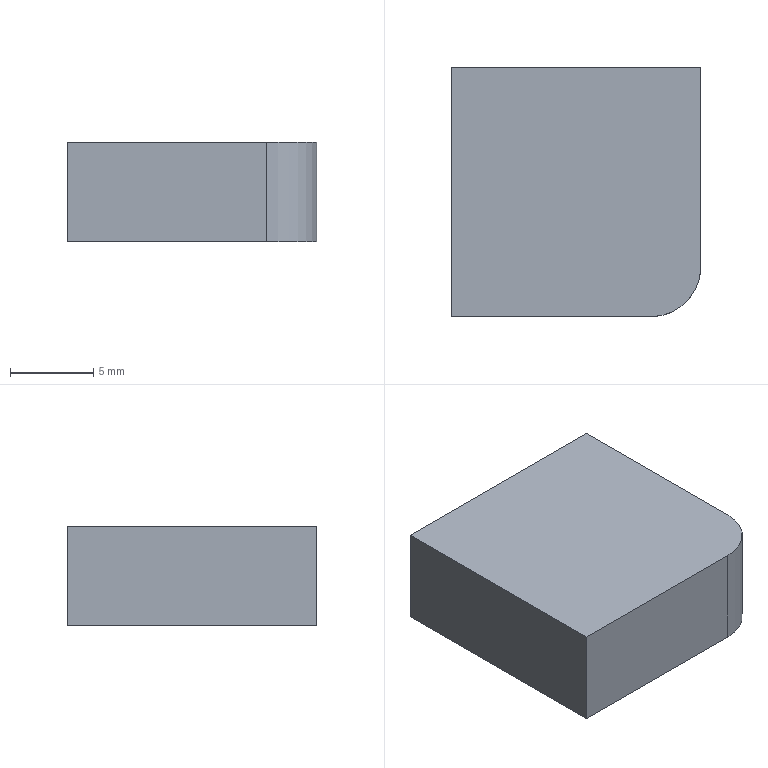Part | SolidWorks | features FlatPattern 1, SMBaseFlange 1, SheetMetal 1 | 1 solid | 7 faces | box 15 x 15 x 6 mm | volume 1338 mm3 | plane 6 | cylinder 1 | commonest cylinder face diameters 6 x1
STEP:
#1=CARTESIAN_POINT('',(675.3,-99.409,0.));
#2=VERTEX_POINT('',#1);
#3=CARTESIAN_POINT('',(675.3,-87.409,0.));
#4=VERTEX_POINT('',#3);
#5=CARTESIAN_POINT('',(675.3,-87.409,0.));
#6=DIRECTION('',(0.,1.,0.));
#7=VECTOR('',#6,1000.);
#8=LINE('',#5,#7);
#9=EDGE_CURVE('',#2,#4,#8,.T.);
#10=ORIENTED_EDGE('',*,*,#9,.F.);
#11=CARTESIAN_POINT('',(675.3,-99.409,-6.));
#12=VERTEX_POINT('',#11);
#13=CARTESIAN_POINT('',(675.3,-99.409,-6.));
#14=DIRECTION('',(0.,0.,1.));
#15=VECTOR('',#14,1000.);
#16=LINE('',#13,#15);
#17=EDGE_CURVE('',#12,#2,#16,.T.);
#18=ORIENTED_EDGE('',*,*,#17,.F.);
#19=CARTESIAN_POINT('',(675.3,-87.409,-6.));
#20=VERTEX_POINT('',#19);
#21=CARTESIAN_POINT('',(675.3,-87.409,-6.));
#22=DIRECTION('',(0.,1.,0.));
#23=VECTOR('',#22,1000.);
#24=LINE('',#21,#23);
#25=EDGE_CURVE('',#12,#20,#24,.T.);
#26=ORIENTED_EDGE('',*,*,#25,.T.);
#27=CARTESIAN_POINT('',(675.3,-87.409,-6.));
#28=DIRECTION('',(0.,0.,1.));
#29=VECTOR('',#28,1000.);
#30=LINE('',#27,#29);
#31=EDGE_CURVE('',#20,#4,#30,.T.);
#32=ORIENTED_EDGE('',*,*,#31,.T.);
#33=EDGE_LOOP('',(#10,#18,#26,#32));
#34=FACE_OUTER_BOUND('',#33,.T.);
#35=CARTESIAN_POINT('',(675.3,-87.409,-6.));
#36=DIRECTION('',(1.,0.,0.));
#37=DIRECTION('',(0.,0.,-1.));
#38=AXIS2_PLACEMENT_3D('',#35,#36,#37);
#39=PLANE('',#38);
#40=ADVANCED_FACE('',(#34),#39,.T.);
#41=CARTESIAN_POINT('',(672.3,-102.409,0.));
#42=VERTEX_POINT('',#41);
#43=CARTESIAN_POINT('',(672.3,-99.409,0.));
#44=DIRECTION('',(0.,0.,1.));
#45=DIRECTION('',(-1.,0.,0.));
#46=AXIS2_PLACEMENT_3D('',#43,#44,#45);
#47=CIRCLE('',#46,3.);
#48=EDGE_CURVE('',#42,#2,#47,.T.);
#49=ORIENTED_EDGE('',*,*,#48,.F.);
#50=CARTESIAN_POINT('',(672.3,-102.409,-6.));
#51=VERTEX_POINT('',#50);
#52=CARTESIAN_POINT('',(672.3,-102.409,-6.));
#53=DIRECTION('',(0.,0.,1.));
#54=VECTOR('',#53,1000.);
#55=LINE('',#52,#54);
#56=EDGE_CURVE('',#51,#42,#55,.T.);
#57=ORIENTED_EDGE('',*,*,#56,.F.);
#58=CARTESIAN_POINT('',(672.3,-99.409,-6.));
#59=DIRECTION('',(0.,0.,1.));
#60=DIRECTION('',(-1.,0.,0.));
#61=AXIS2_PLACEMENT_3D('',#58,#59,#60);
#62=CIRCLE('',#61,3.);
#63=EDGE_CURVE('',#51,#12,#62,.T.);
#64=ORIENTED_EDGE('',*,*,#63,.T.);
#65=ORIENTED_EDGE('',*,*,#17,.T.);
#66=EDGE_LOOP('',(#49,#57,#64,#65));
#67=FACE_OUTER_BOUND('',#66,.T.);
#68=CARTESIAN_POINT('',(672.3,-99.409,-6.));
#69=DIRECTION('',(0.,0.,1.));
#70=DIRECTION('',(1.,0.,0.));
#71=AXIS2_PLACEMENT_3D('',#68,#69,#70);
#72=CYLINDRICAL_SURFACE('',#71,3.);
#73=ADVANCED_FACE('',(#67),#72,.T.);
#74=CARTESIAN_POINT('',(660.3,-102.409,0.));
#75=VERTEX_POINT('',#74);
#76=CARTESIAN_POINT('',(672.3,-102.409,0.));
#77=DIRECTION('',(1.,0.,0.));
#78=VECTOR('',#77,1000.);
#79=LINE('',#76,#78);
#80=EDGE_CURVE('',#75,#42,#79,.T.);
#81=ORIENTED_EDGE('',*,*,#80,.F.);
#82=CARTESIAN_POINT('',(660.3,-102.409,-6.));
#83=VERTEX_POINT('',#82);
#84=CARTESIAN_POINT('',(660.3,-102.409,-6.));
#85=DIRECTION('',(0.,0.,1.));
#86=VECTOR('',#85,1000.);
#87=LINE('',#84,#86);
#88=EDGE_CURVE('',#83,#75,#87,.T.);
#89=ORIENTED_EDGE('',*,*,#88,.F.);
#90=CARTESIAN_POINT('',(672.3,-102.409,-6.));
#91=DIRECTION('',(1.,0.,0.));
#92=VECTOR('',#91,1000.);
#93=LINE('',#90,#92);
#94=EDGE_CURVE('',#83,#51,#93,.T.);
#95=ORIENTED_EDGE('',*,*,#94,.T.);
#96=ORIENTED_EDGE('',*,*,#56,.T.);
#97=EDGE_LOOP('',(#81,#89,#95,#96));
#98=FACE_OUTER_BOUND('',#97,.T.);
#99=CARTESIAN_POINT('',(672.3,-102.409,-6.));
#100=DIRECTION('',(0.,-1.,0.));
#101=DIRECTION('',(0.,0.,-1.));
#102=AXIS2_PLACEMENT_3D('',#99,#100,#101);
#103=PLANE('',#102);
#104=ADVANCED_FACE('',(#98),#103,.T.);
#105=CARTESIAN_POINT('',(660.3,-87.409,0.));
#106=VERTEX_POINT('',#105);
#107=CARTESIAN_POINT('',(660.3,-87.409,0.));
#108=DIRECTION('',(0.,-1.,0.));
#109=VECTOR('',#108,1000.);
#110=LINE('',#107,#109);
#111=EDGE_CURVE('',#106,#75,#110,.T.);
#112=ORIENTED_EDGE('',*,*,#111,.F.);
#113=CARTESIAN_POINT('',(660.3,-87.409,-6.));
#114=VERTEX_POINT('',#113);
#115=CARTESIAN_POINT('',(660.3,-87.409,-6.));
#116=DIRECTION('',(0.,0.,1.));
#117=VECTOR('',#116,1000.);
#118=LINE('',#115,#117);
#119=EDGE_CURVE('',#114,#106,#118,.T.);
#120=ORIENTED_EDGE('',*,*,#119,.F.);
#121=CARTESIAN_POINT('',(660.3,-87.409,-6.));
#122=DIRECTION('',(0.,-1.,0.));
#123=VECTOR('',#122,1000.);
#124=LINE('',#121,#123);
#125=EDGE_CURVE('',#114,#83,#124,.T.);
#126=ORIENTED_EDGE('',*,*,#125,.T.);
#127=ORIENTED_EDGE('',*,*,#88,.T.);
#128=EDGE_LOOP('',(#112,#120,#126,#127));
#129=FACE_OUTER_BOUND('',#128,.T.);
#130=CARTESIAN_POINT('',(660.3,-87.409,-6.));
#131=DIRECTION('',(-1.,0.,0.));
#132=DIRECTION('',(0.,-1.,0.));
#133=AXIS2_PLACEMENT_3D('',#130,#131,#132);
#134=PLANE('',#133);
#135=ADVANCED_FACE('',(#129),#134,.T.);
#136=CARTESIAN_POINT('',(675.3,-87.409,0.));
#137=DIRECTION('',(-1.,0.,0.));
#138=VECTOR('',#137,1000.);
#139=LINE('',#136,#138);
#140=EDGE_CURVE('',#4,#106,#139,.T.);
#141=ORIENTED_EDGE('',*,*,#140,.F.);
#142=ORIENTED_EDGE('',*,*,#31,.F.);
#143=CARTESIAN_POINT('',(675.3,-87.409,-6.));
#144=DIRECTION('',(-1.,0.,0.));
#145=VECTOR('',#144,1000.);
#146=LINE('',#143,#145);
#147=EDGE_CURVE('',#20,#114,#146,.T.);
#148=ORIENTED_EDGE('',*,*,#147,.T.);
#149=ORIENTED_EDGE('',*,*,#119,.T.);
#150=EDGE_LOOP('',(#141,#142,#148,#149));
#151=FACE_OUTER_BOUND('',#150,.T.);
#152=CARTESIAN_POINT('',(675.3,-87.409,-6.));
#153=DIRECTION('',(0.,1.,0.));
#154=DIRECTION('',(-1.,0.,0.));
#155=AXIS2_PLACEMENT_3D('',#152,#153,#154);
#156=PLANE('',#155);
#157=ADVANCED_FACE('',(#151),#156,.T.);
#158=ORIENTED_EDGE('',*,*,#25,.F.);
#159=ORIENTED_EDGE('',*,*,#63,.F.);
#160=ORIENTED_EDGE('',*,*,#94,.F.);
#161=ORIENTED_EDGE('',*,*,#125,.F.);
#162=ORIENTED_EDGE('',*,*,#147,.F.);
#163=EDGE_LOOP('',(#158,#159,#160,#161,#162));
#164=FACE_OUTER_BOUND('',#163,.T.);
#165=CARTESIAN_POINT('',(672.3,-99.409,-6.));
#166=DIRECTION('',(0.,0.,-1.));
#167=DIRECTION('',(-1.,0.,0.));
#168=AXIS2_PLACEMENT_3D('',#165,#166,#167);
#169=PLANE('',#168);
#170=ADVANCED_FACE('',(#164),#169,.T.);
#171=ORIENTED_EDGE('',*,*,#9,.T.);
#172=ORIENTED_EDGE('',*,*,#140,.T.);
#173=ORIENTED_EDGE('',*,*,#111,.T.);
#174=ORIENTED_EDGE('',*,*,#80,.T.);
#175=ORIENTED_EDGE('',*,*,#48,.T.);
#176=EDGE_LOOP('',(#171,#172,#173,#174,#175));
#177=FACE_OUTER_BOUND('',#176,.T.);
#178=CARTESIAN_POINT('',(672.3,-99.409,0.));
#179=DIRECTION('',(0.,0.,-1.));
#180=DIRECTION('',(-1.,0.,0.));
#181=AXIS2_PLACEMENT_3D('',#178,#179,#180);
#182=PLANE('',#181);
#183=ADVANCED_FACE('',(#177),#182,.F.);
#184=CLOSED_SHELL('',(#40,#73,#104,#135,#157,#170,#183));
#185=MANIFOLD_SOLID_BREP('',#184);
#186=CARTESIAN_POINT('',(0.,0.,0.));
#187=DIRECTION('',(0.,0.,1.));
#188=DIRECTION('',(1.,0.,0.));
#189=AXIS2_PLACEMENT_3D('',#186,#187,#188);
#190=(LENGTH_UNIT()NAMED_UNIT(*)SI_UNIT(.MILLI.,.METRE.));
#191=UNCERTAINTY_MEASURE_WITH_UNIT(LENGTH_MEASURE(0.00001),#190,'','');
#192=(NAMED_UNIT(*)PLANE_ANGLE_UNIT()SI_UNIT($,.RADIAN.));
#193=(NAMED_UNIT(*)SI_UNIT($,.STERADIAN.)SOLID_ANGLE_UNIT());
#194=(GEOMETRIC_REPRESENTATION_CONTEXT(3)GLOBAL_UNCERTAINTY_ASSIGNED_CONTEXT((#191))GLOBAL_UNIT_ASSIGNED_CONTEXT((#190,#192,#193))REPRESENTATION_CONTEXT('',''));
#195=ADVANCED_BREP_SHAPE_REPRESENTATION('',(#185,#189),#194);